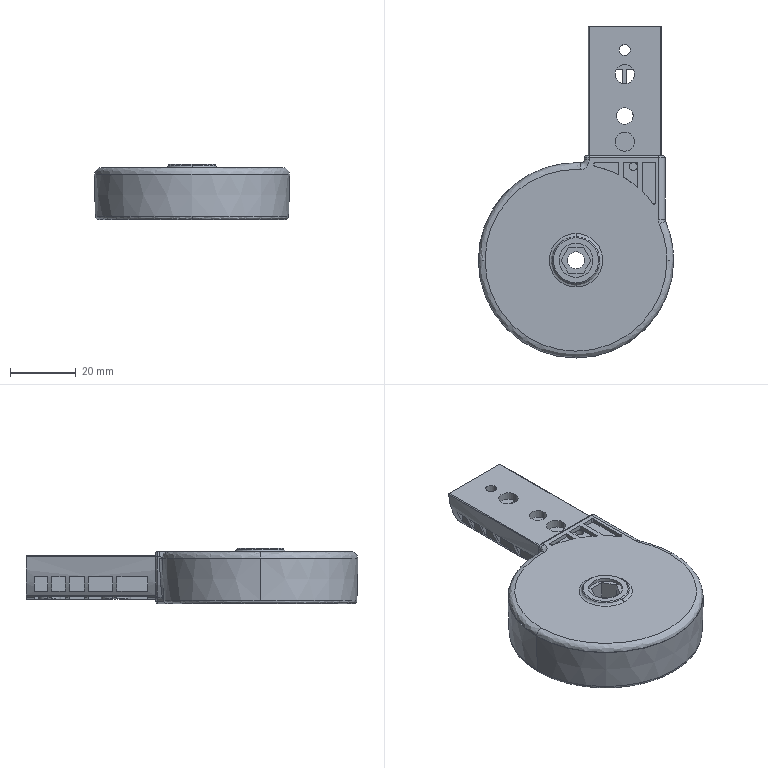Part | SolidWorks | features BaseBody 1 | 1 solid | 301 faces | box 59.608 x 101.264 x 16.804 mm | volume 29040 mm3 | plane 163 | cylinder 89 | spline 43 | cone 6 | commonest cylinder face diameters 53.372 x17 44.411 x9 39.509 x7 5.149 x6 5.882 x6 1.961 x5